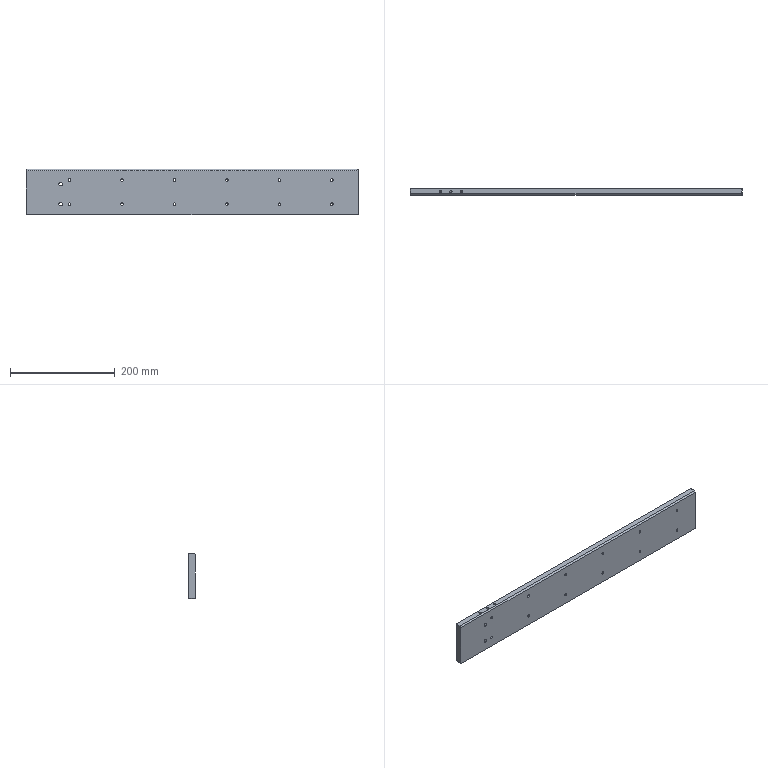Part | SolidWorks | features HoleWzd 6, Cut 5, ICE 3, Chamfer 2, LPattern 2, Extrusion 1 | 1 solid | 95 faces | box 633 x 12 x 86.5 mm | volume 646529 mm3 | cylinder 57 | cone 22 | plane 16 | commonest cylinder face diameters 5 x43 4.2 x6 6.6 x4 11 x4